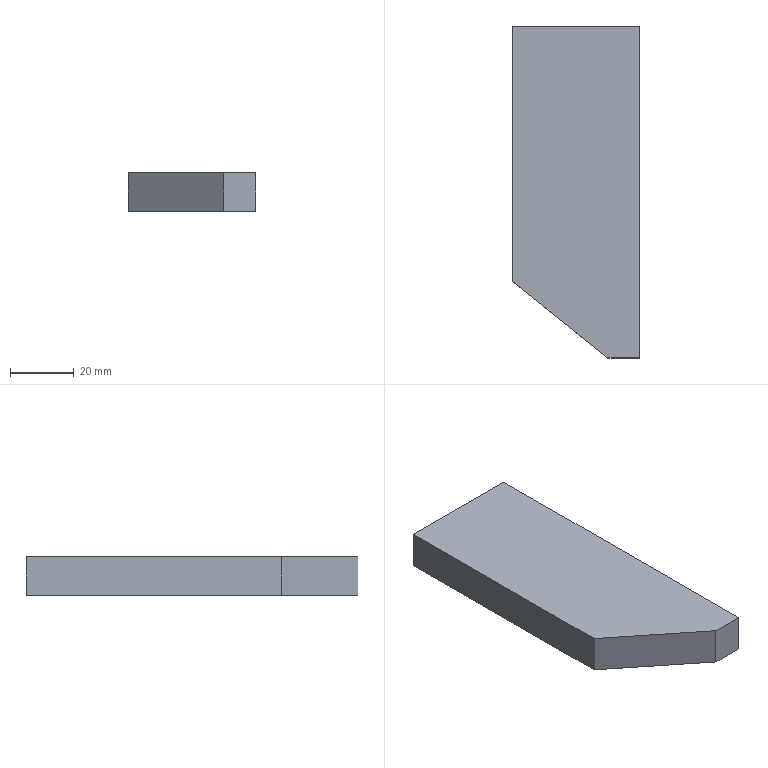Part | SolidWorks | features ICE 2, Extrusion 1 | 1 solid | 7 faces | box 40 x 104 x 12 mm | volume 45600 mm3 | plane 7
STEP:
#1=CARTESIAN_POINT('',(-62.5,-155.,6.));
#2=VERTEX_POINT('',#1);
#3=CARTESIAN_POINT('',(-62.5,-155.,-6.));
#4=VERTEX_POINT('',#3);
#5=CARTESIAN_POINT('',(-62.5,-155.,6.));
#6=DIRECTION('',(0.,0.,-1.));
#7=VECTOR('',#6,1000.);
#8=LINE('',#5,#7);
#9=EDGE_CURVE('',#2,#4,#8,.T.);
#10=ORIENTED_EDGE('',*,*,#9,.F.);
#11=CARTESIAN_POINT('',(-72.5,-155.,6.));
#12=VERTEX_POINT('',#11);
#13=CARTESIAN_POINT('',(-12.5,-155.,6.));
#14=DIRECTION('',(1.,0.,0.));
#15=VECTOR('',#14,1000.);
#16=LINE('',#13,#15);
#17=EDGE_CURVE('',#12,#2,#16,.T.);
#18=ORIENTED_EDGE('',*,*,#17,.F.);
#19=CARTESIAN_POINT('',(-72.5,-155.,-6.));
#20=VERTEX_POINT('',#19);
#21=CARTESIAN_POINT('',(-72.5,-155.,6.));
#22=DIRECTION('',(0.,0.,-1.));
#23=VECTOR('',#22,1000.);
#24=LINE('',#21,#23);
#25=EDGE_CURVE('',#12,#20,#24,.T.);
#26=ORIENTED_EDGE('',*,*,#25,.T.);
#27=CARTESIAN_POINT('',(-12.5,-155.,-6.));
#28=DIRECTION('',(1.,0.,0.));
#29=VECTOR('',#28,1000.);
#30=LINE('',#27,#29);
#31=EDGE_CURVE('',#20,#4,#30,.T.);
#32=ORIENTED_EDGE('',*,*,#31,.T.);
#33=EDGE_LOOP('',(#10,#18,#26,#32));
#34=FACE_OUTER_BOUND('',#33,.T.);
#35=CARTESIAN_POINT('',(-12.5,-155.,6.));
#36=DIRECTION('',(0.,1.,0.));
#37=DIRECTION('',(0.,0.,1.));
#38=AXIS2_PLACEMENT_3D('',#35,#36,#37);
#39=PLANE('',#38);
#40=ADVANCED_FACE('',(#34),#39,.F.);
#41=ORIENTED_EDGE('',*,*,#17,.T.);
#42=CARTESIAN_POINT('',(-62.5,-51.,6.));
#43=VERTEX_POINT('',#42);
#44=CARTESIAN_POINT('',(-62.5,-51.,6.));
#45=DIRECTION('',(0.,1.,0.));
#46=VECTOR('',#45,1000.);
#47=LINE('',#44,#46);
#48=EDGE_CURVE('',#2,#43,#47,.T.);
#49=ORIENTED_EDGE('',*,*,#48,.T.);
#50=CARTESIAN_POINT('',(-102.5,-51.,6.));
#51=VERTEX_POINT('',#50);
#52=CARTESIAN_POINT('',(-102.5,-51.,6.));
#53=DIRECTION('',(-1.,0.,0.));
#54=VECTOR('',#53,1000.);
#55=LINE('',#52,#54);
#56=EDGE_CURVE('',#43,#51,#55,.T.);
#57=ORIENTED_EDGE('',*,*,#56,.T.);
#58=CARTESIAN_POINT('',(-102.5,-131.,6.));
#59=VERTEX_POINT('',#58);
#60=CARTESIAN_POINT('',(-102.5,-131.,6.));
#61=DIRECTION('',(0.,-1.,0.));
#62=VECTOR('',#61,1000.);
#63=LINE('',#60,#62);
#64=EDGE_CURVE('',#51,#59,#63,.T.);
#65=ORIENTED_EDGE('',*,*,#64,.T.);
#66=CARTESIAN_POINT('',(-72.5,-155.,6.));
#67=DIRECTION('',(0.7809,-0.6247,0.));
#68=VECTOR('',#67,1000.);
#69=LINE('',#66,#68);
#70=EDGE_CURVE('',#59,#12,#69,.T.);
#71=ORIENTED_EDGE('',*,*,#70,.T.);
#72=EDGE_LOOP('',(#41,#49,#57,#65,#71));
#73=FACE_OUTER_BOUND('',#72,.T.);
#74=CARTESIAN_POINT('',(-12.5,155.,6.));
#75=DIRECTION('',(0.,0.,1.));
#76=DIRECTION('',(1.,0.,0.));
#77=AXIS2_PLACEMENT_3D('',#74,#75,#76);
#78=PLANE('',#77);
#79=ADVANCED_FACE('',(#73),#78,.T.);
#80=CARTESIAN_POINT('',(-62.5,-51.,-6.));
#81=VERTEX_POINT('',#80);
#82=CARTESIAN_POINT('',(-62.5,155.,-6.));
#83=DIRECTION('',(0.,1.,0.));
#84=VECTOR('',#83,1000.);
#85=LINE('',#82,#84);
#86=EDGE_CURVE('',#4,#81,#85,.T.);
#87=ORIENTED_EDGE('',*,*,#86,.F.);
#88=ORIENTED_EDGE('',*,*,#31,.F.);
#89=CARTESIAN_POINT('',(-102.5,-131.,-6.));
#90=VERTEX_POINT('',#89);
#91=CARTESIAN_POINT('',(-72.5,-155.,-6.));
#92=DIRECTION('',(0.7809,-0.6247,0.));
#93=VECTOR('',#92,1000.);
#94=LINE('',#91,#93);
#95=EDGE_CURVE('',#90,#20,#94,.T.);
#96=ORIENTED_EDGE('',*,*,#95,.F.);
#97=CARTESIAN_POINT('',(-102.5,-51.,-6.));
#98=VERTEX_POINT('',#97);
#99=CARTESIAN_POINT('',(-102.5,-131.,-6.));
#100=DIRECTION('',(0.,-1.,0.));
#101=VECTOR('',#100,1000.);
#102=LINE('',#99,#101);
#103=EDGE_CURVE('',#98,#90,#102,.T.);
#104=ORIENTED_EDGE('',*,*,#103,.F.);
#105=CARTESIAN_POINT('',(-102.5,-51.,-6.));
#106=DIRECTION('',(-1.,0.,0.));
#107=VECTOR('',#106,1000.);
#108=LINE('',#105,#107);
#109=EDGE_CURVE('',#81,#98,#108,.T.);
#110=ORIENTED_EDGE('',*,*,#109,.F.);
#111=EDGE_LOOP('',(#87,#88,#96,#104,#110));
#112=FACE_OUTER_BOUND('',#111,.T.);
#113=CARTESIAN_POINT('',(-12.5,155.,-6.));
#114=DIRECTION('',(0.,0.,1.));
#115=DIRECTION('',(1.,0.,0.));
#116=AXIS2_PLACEMENT_3D('',#113,#114,#115);
#117=PLANE('',#116);
#118=ADVANCED_FACE('',(#112),#117,.F.);
#119=CARTESIAN_POINT('',(-62.5,-51.,-16.));
#120=DIRECTION('',(0.,0.,1.));
#121=VECTOR('',#120,1000.);
#122=LINE('',#119,#121);
#123=EDGE_CURVE('',#81,#43,#122,.T.);
#124=ORIENTED_EDGE('',*,*,#123,.F.);
#125=ORIENTED_EDGE('',*,*,#109,.T.);
#126=CARTESIAN_POINT('',(-102.5,-51.,6.));
#127=DIRECTION('',(0.,0.,-1.));
#128=VECTOR('',#127,1000.);
#129=LINE('',#126,#128);
#130=EDGE_CURVE('',#51,#98,#129,.T.);
#131=ORIENTED_EDGE('',*,*,#130,.F.);
#132=ORIENTED_EDGE('',*,*,#56,.F.);
#133=EDGE_LOOP('',(#124,#125,#131,#132));
#134=FACE_OUTER_BOUND('',#133,.T.);
#135=CARTESIAN_POINT('',(-102.5,-51.,6.));
#136=DIRECTION('',(0.,-1.,0.));
#137=DIRECTION('',(1.,0.,0.));
#138=AXIS2_PLACEMENT_3D('',#135,#136,#137);
#139=PLANE('',#138);
#140=ADVANCED_FACE('',(#134),#139,.F.);
#141=ORIENTED_EDGE('',*,*,#103,.T.);
#142=CARTESIAN_POINT('',(-102.5,-131.,6.));
#143=DIRECTION('',(0.,0.,-1.));
#144=VECTOR('',#143,1000.);
#145=LINE('',#142,#144);
#146=EDGE_CURVE('',#59,#90,#145,.T.);
#147=ORIENTED_EDGE('',*,*,#146,.F.);
#148=ORIENTED_EDGE('',*,*,#64,.F.);
#149=ORIENTED_EDGE('',*,*,#130,.T.);
#150=EDGE_LOOP('',(#141,#147,#148,#149));
#151=FACE_OUTER_BOUND('',#150,.T.);
#152=CARTESIAN_POINT('',(-102.5,-131.,6.));
#153=DIRECTION('',(1.,0.,0.));
#154=DIRECTION('',(0.,1.,0.));
#155=AXIS2_PLACEMENT_3D('',#152,#153,#154);
#156=PLANE('',#155);
#157=ADVANCED_FACE('',(#151),#156,.F.);
#158=ORIENTED_EDGE('',*,*,#95,.T.);
#159=ORIENTED_EDGE('',*,*,#25,.F.);
#160=ORIENTED_EDGE('',*,*,#70,.F.);
#161=ORIENTED_EDGE('',*,*,#146,.T.);
#162=EDGE_LOOP('',(#158,#159,#160,#161));
#163=FACE_OUTER_BOUND('',#162,.T.);
#164=CARTESIAN_POINT('',(-72.5,-155.,6.));
#165=DIRECTION('',(0.6247,0.7809,0.));
#166=DIRECTION('',(-0.7809,0.6247,0.));
#167=AXIS2_PLACEMENT_3D('',#164,#165,#166);
#168=PLANE('',#167);
#169=ADVANCED_FACE('',(#163),#168,.F.);
#170=ORIENTED_EDGE('',*,*,#9,.T.);
#171=ORIENTED_EDGE('',*,*,#86,.T.);
#172=ORIENTED_EDGE('',*,*,#123,.T.);
#173=ORIENTED_EDGE('',*,*,#48,.F.);
#174=EDGE_LOOP('',(#170,#171,#172,#173));
#175=FACE_OUTER_BOUND('',#174,.T.);
#176=CARTESIAN_POINT('',(-62.5,-51.,-16.));
#177=DIRECTION('',(1.,0.,0.));
#178=DIRECTION('',(0.,1.,0.));
#179=AXIS2_PLACEMENT_3D('',#176,#177,#178);
#180=PLANE('',#179);
#181=ADVANCED_FACE('',(#175),#180,.T.);
#182=CLOSED_SHELL('',(#40,#79,#118,#140,#157,#169,#181));
#183=MANIFOLD_SOLID_BREP('',#182);
#184=CARTESIAN_POINT('',(0.,0.,0.));
#185=DIRECTION('',(0.,0.,1.));
#186=DIRECTION('',(1.,0.,0.));
#187=AXIS2_PLACEMENT_3D('',#184,#185,#186);
#188=(LENGTH_UNIT()NAMED_UNIT(*)SI_UNIT(.MILLI.,.METRE.));
#189=UNCERTAINTY_MEASURE_WITH_UNIT(LENGTH_MEASURE(0.00001),#188,'','');
#190=(NAMED_UNIT(*)PLANE_ANGLE_UNIT()SI_UNIT($,.RADIAN.));
#191=(NAMED_UNIT(*)SI_UNIT($,.STERADIAN.)SOLID_ANGLE_UNIT());
#192=(GEOMETRIC_REPRESENTATION_CONTEXT(3)GLOBAL_UNCERTAINTY_ASSIGNED_CONTEXT((#189))GLOBAL_UNIT_ASSIGNED_CONTEXT((#188,#190,#191))REPRESENTATION_CONTEXT('',''));
#193=ADVANCED_BREP_SHAPE_REPRESENTATION('',(#183,#187),#192);